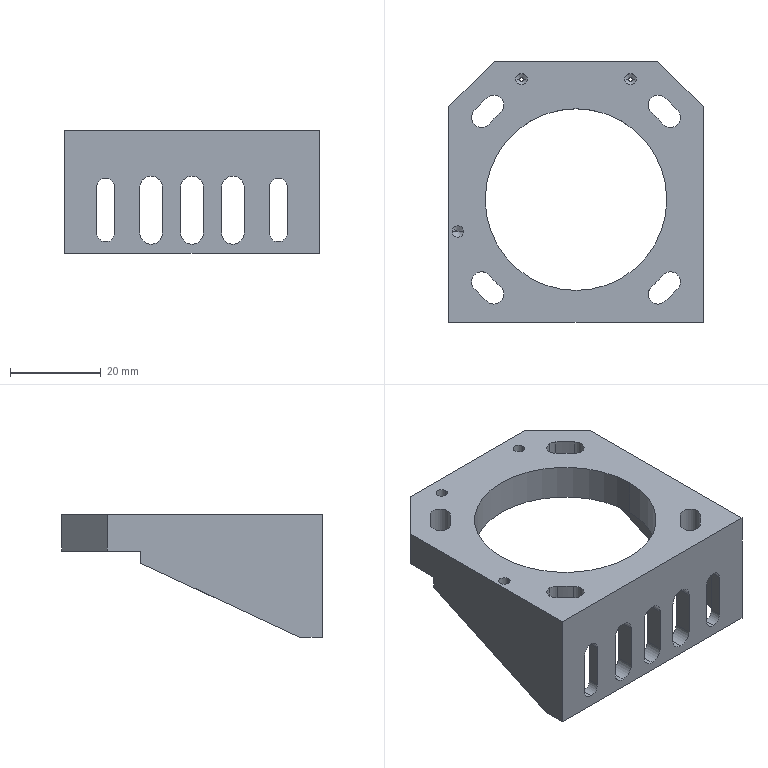NC program | NX | posted with a generic post | part box 56 x 57.4 x 27 mm
Lines 19681 to 20877 of 23725:
(ZLEVEL_PROFILE_COPY_2_COPY_COPY , TOOL : D6R0.5)
N39330 T05 M6
N39332 G54
N39334 G17 G0 G90 X-19.929 Y-23.487 B0. C0. S7000 M3
N39336 G43 Z30. H5
N39338 Z0.958
N39340 G94 G1 Z-0.042 F1000.
N39342 X-20.699 Y-23.932
N39344 G3 X-20.999 Y-24.451 R0.6
N39346 G1 Y-28.473 F3000.
N39348 X-20.953 Y-28.474 Z-0.063
N39350 X-20.909 Z-0.085
N39352 X-20.908 Y-28.
N39354 Y-24.969
N39356 Y-24.456
N39358 X-20.863 Y-24.459 Z-0.106
N39360 X-20.818 Y-24.461 Z-0.127
N39362 X-20.817 Y-24.98
N39364 Y-28.
N39366 X-20.818 Y-28.475
N39368 X-20.772 Z-0.148
N39370 X-20.727 Z-0.169
N39372 Y-28.
N39374 Y-24.99
N39376 Y-24.464
N39378 X-20.681 Y-24.466 Z-0.19
N39380 X-20.637 Y-24.467 Z-0.211
N39382 X-20.636 Y-24.994
N39384 Y-28.
N39386 X-20.637 Y-28.476
N39388 X-20.591 Z-0.232
N39390 X-20.546 Z-0.254
N39392 X-20.545 Y-28.
N39394 Y-24.998
N39396 X-20.546 Y-24.47
N39398 X-20.5 Y-24.471 Z-0.275
N39400 X-20.455 Y-24.472 Z-0.296
N39402 Y-25.
N39404 Y-28.
N39406 Y-28.477
N39408 X-20.409 Z-0.317
N39410 X-20.365 Y-28.478 Z-0.338
N39412 X-20.364 Y-28.
N39414 Y-25.
N39416 X-20.365 Y-24.473
N39418 X-20.319 Y-24.474 Z-0.359
N39420 X-20.274 Z-0.38
N39422 X-20.273 Y-25.
N39424 Y-28.
N39426 X-20.274 Y-28.478
N39428 X-20.228 Z-0.401
N39430 X-20.184 Y-28.479 Z-0.423
N39432 X-20.183 Y-28.
N39434 Y-25.
N39436 X-20.184 Y-24.475
N39438 X-20.138 Z-0.444
N39440 X-20.093 Z-0.465
N39442 X-20.092 Y-25.
N39444 Y-28.
N39446 X-20.093 Y-28.479
N39448 X-20.047 Y-28.48 Z-0.486
N39450 X-20.002 Z-0.507
N39452 Y-28.
N39454 Y-25.
N39456 Y-24.476
N39458 X-19.956 Y-24.477 Z-0.528
N39460 X-19.912 Z-0.549
N39462 X-19.911 Y-25.
N39464 Y-28.
N39466 X-19.912 Y-28.48
N39468 X-19.866 Y-28.481 Z-0.571
N39470 X-19.821 Z-0.592
N39472 X-19.82 Y-28.
N39474 Y-25.
N39476 X-19.821 Y-24.478
N39478 X-19.775 Z-0.613
N39480 X-19.731 Z-0.634
N39482 X-19.73 Y-25.
N39484 Y-28.
N39486 Y-28.482
N39488 X-19.684 Z-0.655
N39490 X-19.64 Z-0.676
N39492 X-19.639 Y-28.
N39494 Y-25.
N39496 X-19.64 Y-24.479
N39498 X-19.594 Y-24.48 Z-0.697
N39500 X-19.549 Z-0.718
N39502 X-19.548 Y-25.
N39504 Y-28.
N39506 X-19.549 Y-28.483
N39508 X-19.503 Z-0.74
N39510 X-19.458 Z-0.761
N39512 Y-28.
N39514 Y-25.
N39516 X-19.459 Y-24.481
N39518 X-19.412 Z-0.782
N39520 X-19.368 Z-0.803
N39522 X-19.367 Y-25.
N39524 Y-28.
N39526 X-19.368 Y-28.484
N39528 X-19.322 Z-0.824
N39530 X-19.277 Z-0.845
N39532 Y-28.
N39534 Y-25.
N39536 Y-24.482
N39538 X-19.231 Z-0.866
N39540 X-19.187 Y-24.483 Z-0.887
N39542 X-19.186 Y-25.
N39544 Y-28.
N39546 Y-28.485
N39548 X-19.141 Z-0.909
N39550 X-19.096 Z-0.93
N39552 X-19.095 Y-28.
N39554 Y-25.
N39556 X-19.096 Y-24.483
N39558 X-19.05 Y-24.484 Z-0.951
N39560 X-19.006 Z-0.972
N39562 X-19.005 Y-25.
N39564 Y-28.
N39566 Y-28.486
N39568 X-18.959 Z-0.993
N39570 X-18.915 Z-1.014
N39572 X-18.914 Y-28.
N39574 Y-25.
N39576 X-18.915 Y-24.485
N39578 X-18.869 Z-1.035
N39580 X-18.824 Y-24.486 Z-1.057
N39582 X-18.823 Y-25.
N39584 Y-28.
N39586 X-18.824 Y-28.487
N39588 X-18.778 Z-1.078
N39590 X-18.733 Z-1.099
N39592 Y-28.
N39594 Y-25.
N39596 X-18.734 Y-24.486
N39598 X-18.687 Z-1.12
N39600 X-18.643 Y-24.487 Z-1.141
N39602 X-18.642 Y-25.
N39604 Y-28.
N39606 X-18.643 Y-28.487
N39608 X-18.597 Y-28.488 Z-1.162
N39610 X-18.552 Z-1.183
N39612 X-18.551 Y-28.
N39614 Y-25.
N39616 X-18.553 Y-24.487
N39618 X-18.506 Z-1.204
N39620 X-18.462 Z-1.226
N39622 X-18.461 Y-25.
N39624 Y-28.
N39626 Y-28.488
N39628 X-18.416 Y-28.489 Z-1.247
N39630 X-18.371 Z-1.268
N39632 X-18.37 Y-28.
N39634 Y-25.
N39636 X-18.371 Y-24.488
N39638 X-18.325 Z-1.289
N39640 X-18.281 Z-1.31
N39642 X-18.28 Y-25.
N39644 Y-28.
N39646 Y-28.489
N39648 X-18.234 Z-1.331
N39650 X-18.189 Y-28.49 Z-1.352
N39652 Y-28.
N39654 Y-25.
N39656 X-18.19 Y-24.489
N39658 X-18.144 Z-1.374
N39660 X-18.099 Z-1.395
N39662 X-18.098 Y-25.
N39664 Y-28.
N39666 X-18.099 Y-28.49
N39668 X-18.053 Z-1.416
N39670 X-18.008 Y-28.491 Z-1.437
N39672 Y-28.
N39674 Y-25.
N39676 X-18.009 Y-24.49
N39678 X-17.962 Z-1.458
N39680 X-17.918 Z-1.479
N39682 X-17.917 Y-25.
N39684 Y-28.
N39686 X-17.918 Y-28.491
N39688 X-17.872 Z-1.5
N39690 X-17.827 Z-1.521
N39692 X-17.826 Y-28.
N39694 Y-25.
N39696 X-17.828 Y-24.49
N39698 X-17.781 Y-24.491 Z-1.543
N39700 X-17.737 Z-1.564
N39702 X-17.736 Y-25.
N39704 Y-28.
N39706 Y-28.492
N39708 X-17.69 Z-1.585
N39710 X-17.646 Z-1.606
N39712 X-17.645 Y-28.
N39714 Y-25.
N39716 X-17.646 Y-24.491
N39718 X-17.6 Z-1.627
N39720 X-17.556 Y-24.492 Z-1.648
N39722 X-17.555 Y-25.
N39724 Y-28.
N39726 Y-28.493
N39728 X-17.509 Z-1.669
N39730 X-17.464 Z-1.69
N39732 Y-28.
N39734 Y-25.
N39736 X-17.465 Y-24.492
N39738 X-17.419 Z-1.712
N39740 X-17.374 Z-1.733
N39742 X-17.373 Y-25.
N39744 Y-28.
N39746 X-17.374 Y-28.493
N39748 X-17.328 Z-1.754
N39750 X-17.283 Z-1.775
N39752 Y-28.
N39754 Y-25.
N39756 X-17.284 Y-24.493
N39758 X-17.237 Z-1.796
N39760 X-17.193 Z-1.817
N39762 X-17.192 Y-25.
N39764 Y-28.
N39766 Y-28.494
N39768 X-17.147 Z-1.838
N39770 X-17.102 Z-1.86
N39772 X-17.101 Y-28.
N39774 Y-25.
N39776 X-17.103 Y-24.494
N39778 X-17.056 Z-1.881
N39780 X-17.012 Z-1.902
N39782 X-17.011 Y-25.
N39784 Y-28.
N39786 Y-28.494
N39788 X-16.965 Z-1.923
N39790 X-16.921 Z-1.944
N39792 X-16.92 Y-28.
N39794 Y-25.
N39796 X-16.921 Y-24.494
N39798 X-16.875 Z-1.965
N39800 X-16.831 Y-24.495 Z-1.986
N39802 X-16.83 Y-25.
N39804 Y-28.
N39806 Y-28.495
N39808 X-16.784 Z-2.007
N39810 X-16.739 Z-2.029
N39812 Y-28.
N39814 Y-25.
N39816 X-16.74 Y-24.495
N39818 X-16.694 Z-2.05
N39820 X-16.649 Z-2.071
N39822 X-16.648 Y-25.
N39824 Y-28.
N39826 X-16.649 Y-28.495
N39828 X-16.603 Z-2.092
N39830 X-16.558 Z-2.113
N39832 Y-28.
N39834 Y-25.
N39836 X-16.559 Y-24.495
N39838 X-16.512 Z-2.134
N39840 X-16.468 Z-2.155
N39842 X-16.467 Y-25.
N39844 Y-28.
N39846 Y-28.495
N39848 X-16.422 Z-2.176
N39850 X-16.377 Y-28.496 Z-2.198
N39852 X-16.376 Y-28.
N39854 Y-25.
N39856 X-16.378 Y-24.495
N39858 X-16.331 Y-24.496 Z-2.219
N39860 X-16.287 Z-2.24
N39862 X-16.286 Y-25.
N39864 Y-28.
N39866 Y-28.496
N39868 X-16.24 Z-2.261
N39870 X-16.196 Z-2.282
N39872 X-16.195 Y-28.
N39874 Y-25.
N39876 X-16.196 Y-24.496
N39878 X-16.15 Z-2.303
N39880 X-16.106 Z-2.324
N39882 X-16.104 Y-25.
N39884 Y-28.
N39886 X-16.105 Y-28.496
N39888 X-16.059 Z-2.346
N39890 X-16.014 Y-28.497 Z-2.367
N39892 Y-28.
N39894 Y-25.
N39896 X-16.015 Y-24.496
N39898 X-15.969 Y-24.497 Z-2.388
N39900 X-15.924 Z-2.409
N39902 X-15.923 Y-25.
N39904 Y-28.
N39906 X-15.924 Y-28.497
N39908 X-15.878 Z-2.43
N39910 X-15.833 Z-2.451
N39912 Y-28.
N39914 Y-25.
N39916 X-15.834 Y-24.497
N39918 X-15.787 Z-2.472
N39920 X-15.743 Z-2.493
N39922 X-15.742 Y-25.
N39924 Y-28.
N39926 Y-28.497
N39928 X-15.697 Z-2.515
N39930 X-15.652 Z-2.536
N39932 X-15.651 Y-28.
N39934 Y-25.
N39936 X-15.653 Y-24.497
N39938 X-15.606 Z-2.557
N39940 X-15.562 Z-2.578
N39942 X-15.561 Y-25.
N39944 Y-28.
N39946 Y-28.497
N39948 X-15.515 Z-2.599
N39950 X-15.47 Z-2.62
N39952 Y-28.
N39954 Y-25.
N39956 X-15.471 Y-24.498
N39958 X-15.425 Z-2.641
N39960 X-15.381 Z-2.662
N39962 X-15.379 Y-25.
N39964 Y-28.
N39966 X-15.38 Y-28.498
N39968 X-15.334 Z-2.684
N39970 X-15.289 Z-2.705
N39972 Y-28.
N39974 Y-25.
N39976 X-15.29 Y-24.498
N39978 X-15.243 Z-2.726
N39980 X-15.199 Z-2.747
N39982 X-15.198 Y-25.
N39984 Y-28.
N39986 X-15.199 Y-28.498
N39988 X-15.153 Z-2.768
N39990 X-15.108 Z-2.789
N39992 Y-28.
N39994 Y-25.
N39996 X-15.109 Y-24.498
N39998 X-15.062 Z-2.81
N40000 X-15.018 Z-2.832
N40002 X-15.017 Y-25.
N40004 Y-28.
N40006 Y-28.498
N40008 X-14.972 Z-2.853
N40010 X-14.927 Z-2.874
N40012 X-14.926 Y-28.
N40014 Y-25.
N40016 X-14.927 Y-24.498
N40018 X-14.881 Z-2.895
N40020 X-14.837 Z-2.916
N40022 X-14.836 Y-25.
N40024 Y-28.
N40026 Y-28.498
N40028 X-14.79 Z-2.937
N40030 X-14.745 Z-2.958
N40032 Y-28.
N40034 Y-25.
N40036 X-14.746 Y-24.498
N40038 X-14.7 Z-2.979
N40040 X-14.656 Z-3.001
N40042 X-14.654 Y-25.
N40044 Y-28.
N40046 X-14.655 Y-28.498
N40048 X-14.609 Z-3.022
N40050 X-14.564 Z-3.043
N40052 Y-28.
N40054 Y-25.
N40056 X-14.565 Y-24.499
N40058 X-14.518 Z-3.064
N40060 X-14.474 Z-3.085
N40062 X-14.473 Y-25.
N40064 Y-28.
N40066 Y-28.498
N40068 X-14.428 Y-28.499 Z-3.106
N40070 X-14.383 Z-3.127
N40072 X-14.382 Y-28.
N40074 Y-25.
N40076 X-14.384 Y-24.499
N40078 X-14.337 Z-3.149
N40080 X-14.293 Z-3.17
N40082 X-14.292 Y-25.
N40084 Y-28.
N40086 Y-28.499
N40088 X-14.247 Z-3.191
N40090 X-14.202 Z-3.212
N40092 X-14.201 Y-28.
N40094 Y-25.
N40096 X-14.202 Y-24.499
N40098 X-14.156 Z-3.233
N40100 X-14.112 Z-3.254
N40102 X-14.111 Y-25.
N40104 Y-28.
N40106 Y-28.499
N40108 X-14.065 Z-3.275
N40110 X-14.02 Z-3.296
N40112 Y-28.
N40114 Y-25.
N40116 X-14.021 Y-24.499
N40118 X-13.975 Z-3.318
N40120 X-13.931 Z-3.339
N40122 X-13.929 Y-25.
N40124 Y-28.
N40126 X-13.93 Y-28.499
N40128 X-13.884 Z-3.36
N40130 X-13.839 Z-3.381
N40132 Y-28.
N40134 Y-25.
N40136 X-13.84 Y-24.499
N40138 X-13.793 Z-3.402
N40140 X-13.749 Z-3.423
N40142 X-13.748 Y-25.
N40144 Y-28.
N40146 Y-28.499
N40148 X-13.703 Z-3.444
N40150 X-13.658 Z-3.465
N40152 X-13.657 Y-28.
N40154 Y-25.
N40156 X-13.659 Y-24.499
N40158 X-13.612 Z-3.487
N40160 X-13.568 Z-3.508
N40162 X-13.567 Y-25.
N40164 Y-28.
N40166 Y-28.499
N40168 X-13.521 Z-3.529
N40170 X-13.477 Z-3.55
N40172 X-13.476 Y-28.
N40174 Y-25.
N40176 X-13.477 Y-24.499
N40178 X-13.431 Z-3.571
N40180 X-13.387 Z-3.592
N40182 X-13.386 Y-25.
N40184 Y-28.
N40186 Y-28.499
N40188 X-13.34 Z-3.613
N40190 X-13.295 Z-3.635
N40192 Y-28.
N40194 Y-25.
N40196 X-13.296 Y-24.499
N40198 X-13.25 Z-3.656
N40200 X-13.206 Y-24.5 Z-3.677
N40202 X-13.204 Y-25.
N40204 Y-28.
N40206 X-13.205 Y-28.499
N40208 X-13.159 Z-3.698
N40210 X-13.114 Z-3.719
N40212 Y-28.
N40214 Y-25.
N40216 X-13.115 Y-24.5
N40218 X-13.068 Z-3.74
N40220 X-13.024 Z-3.761
N40222 X-13.023 Y-25.
N40224 Y-28.
N40226 Y-28.499
N40228 X-12.978 Z-3.782
N40230 X-12.933 Z-3.804
N40232 X-12.932 Y-28.
N40234 Y-25.
N40236 X-12.934 Y-24.5
N40238 X-12.887 Z-3.825
N40240 X-12.843 Z-3.846
N40242 X-12.842 Y-25.
N40244 Y-28.
N40246 Y-28.499
N40248 X-12.796 Z-3.867
N40250 X-12.751 Z-3.888
N40252 Y-28.
N40254 Y-25.
N40256 X-12.752 Y-24.5
N40258 X-12.706 Z-3.909
N40260 X-12.662 Z-3.93
N40262 X-12.66 Y-25.
N40264 Y-28.
N40266 X-12.661 Y-28.5
N40268 X-12.615 Z-3.951
N40270 X-12.57 Z-3.973
N40272 Y-28.
N40274 Y-25.
N40276 X-12.571 Y-24.5
N40278 X-12.525 Z-3.994
N40280 X-12.48 Z-4.015
N40282 X-12.479 Y-25.
N40284 Y-28.
N40286 X-12.48 Y-28.5
N40288 X-12.434 Z-4.036
N40290 X-12.389 Z-4.057
N40292 Y-28.
N40294 Y-25.
N40296 X-12.39 Y-24.5
N40298 X-12.343 Z-4.078
N40300 X-12.299 Z-4.099
N40302 X-12.298 Y-25.
N40304 Y-28.
N40306 Y-28.5
N40308 X-12.253 Z-4.121
N40310 X-12.208 Z-4.142
N40312 X-12.207 Y-28.
N40314 Y-25.
N40316 X-12.209 Y-24.5
N40318 X-12.162 Z-4.163
N40320 X-12.118 Z-4.184
N40322 X-12.117 Y-25.
N40324 Y-28.
N40326 Y-28.5
N40328 X-12.071 Z-4.205
N40330 X-12.026 Z-4.226
N40332 Y-28.
N40334 Y-25.
N40336 X-12.027 Y-24.5
N40338 X-11.981 Z-4.247
N40340 X-11.937 Z-4.268
N40342 X-11.935 Y-25.
N40344 Y-28.
N40346 X-11.936 Y-28.5
N40348 X-11.89 Z-4.29
N40350 X-11.845 Z-4.311
N40352 Y-28.
N40354 Y-25.
N40356 X-11.846 Y-24.5
N40358 X-11.799 Z-4.332
N40360 X-11.755 Z-4.353
N40362 X-11.754 Y-25.
N40364 Y-28.
N40366 X-11.755 Y-28.5
N40368 X-11.709 Z-4.374
N40370 X-11.664 Z-4.395
N40372 Y-28.
N40374 Y-25.
N40376 X-11.665 Y-24.5
N40378 X-11.618 Z-4.416
N40380 X-11.574 Z-4.437
N40382 X-11.573 Y-25.
N40384 Y-28.
N40386 Y-28.5
N40388 X-11.528 Z-4.459
N40390 X-11.483 Z-4.48
N40392 X-11.482 Y-28.
N40394 Y-25.
N40396 X-11.484 Y-24.5
N40398 X-11.437 Z-4.501
N40400 X-11.393 Z-4.522
N40402 X-11.392 Y-25.
N40404 Y-28.
N40406 Y-28.5
N40408 X-11.346 Z-4.543
N40410 X-11.301 Z-4.564
N40412 Y-28.
N40414 Y-25.
N40416 X-11.302 Y-24.5
N40418 X-11.256 Z-4.585
N40420 X-11.212 Z-4.607
N40422 X-11.21 Y-25.
N40424 Y-28.
N40426 X-11.211 Y-28.5
N40428 X-11.165 Z-4.628
N40430 X-11.12 Z-4.649
N40432 Y-28.
N40434 Y-25.
N40436 X-11.121 Y-24.5
N40438 X-11.074 Z-4.67
N40440 X-11.03 Z-4.691
N40442 X-11.029 Y-25.
N40444 Y-28.
N40446 Y-28.5
N40448 X-10.984 Z-4.712
N40450 X-10.939 Z-4.733
N40452 Y-28.
N40454 Y-25.
N40456 X-10.94 Y-24.5
N40458 X-10.893 Z-4.754
N40460 X-10.849 Z-4.776
N40462 X-10.848 Y-25.
N40464 Y-28.
N40466 Y-28.5
N40468 X-10.803 Z-4.797
N40470 X-10.758 Z-4.818
N40472 X-10.757 Y-28.
N40474 Y-25.
N40476 X-10.759 Y-24.5
N40478 X-10.712 Z-4.839
N40480 X-10.668 Z-4.86
N40482 X-10.667 Y-25.
N40484 Y-28.
N40486 Y-28.5
N40488 X-10.621 Z-4.881
N40490 X-10.576 Z-4.902
N40492 Y-28.
N40494 Y-25.
N40496 X-10.577 Y-24.5
N40498 X-10.531 Z-4.924
N40500 X-10.487 Z-4.945
N40502 X-10.485 Y-25.
N40504 Y-28.
N40506 X-10.486 Y-28.5
N40508 X-10.44 Z-4.966
N40510 X-10.395 Z-4.987
N40512 Y-28.
N40514 Y-25.
N40516 X-10.396 Y-24.5
N40518 X-10.349 Z-5.008
N40520 X-10.305 Z-5.029
N40522 X-10.304 Y-25.
N40524 Y-28.
N40526 Y-28.5
N40528 X-10.259 Z-5.05
N40530 X-10.214 Z-5.071
N40532 X-10.213 Y-28.
N40534 Y-25.
N40536 X-10.215 Y-24.5
N40538 X-10.168 Z-5.093
N40540 X-10.124 Z-5.114
N40542 X-10.123 Y-25.
N40544 Y-28.
N40546 Y-28.5
N40548 X-10.078 Z-5.135
N40550 X-10.033 Z-5.156
N40552 X-10.032 Y-28.
N40554 Y-25.
N40556 X-10.033 Y-24.5
N40558 X-9.987 Z-5.177
N40560 X-9.943 Z-5.198
N40562 X-9.942 Y-25.
N40564 Y-28.
N40566 Y-28.5
N40568 X-9.896 Z-5.219
N40570 X-9.851 Z-5.24
N40572 Y-28.
N40574 Y-25.
N40576 X-9.852 Y-24.5
N40578 X-9.806 Z-5.262
N40580 X-9.762 Z-5.283
N40582 X-9.76 Y-25.
N40584 Y-28.
N40586 X-9.761 Y-28.5
N40588 X-9.715 Z-5.304
N40590 X-9.67 Z-5.325
N40592 Y-28.
N40594 Y-25.
N40596 X-9.671 Y-24.5
N40598 X-9.624 Z-5.346
N40600 X-9.58 Z-5.367
N40602 X-9.579 Y-25.
N40604 Y-28.
N40606 Y-28.5
N40608 X-9.534 Z-5.388
N40610 X-9.489 Z-5.41
N40612 X-9.488 Y-28.
N40614 Y-25.
N40616 X-9.49 Y-24.5
N40618 X-9.443 Z-5.431
N40620 X-9.399 Z-5.452
N40622 X-9.398 Y-25.
N40624 Y-28.
N40626 Y-28.5
N40628 X-9.352 Z-5.473
N40630 X-9.308 Z-5.494
N40632 X-9.307 Y-28.
N40634 Y-25.
N40636 X-9.308 Y-24.5
N40638 X-9.262 Z-5.515
N40640 X-9.218 Z-5.536
N40642 X-9.217 Y-25.
N40644 Y-28.
N40646 Y-28.5
N40648 X-9.171 Z-5.557
N40650 X-9.126 Z-5.579
N40652 Y-28.
N40654 Y-25.
N40656 Y-24.5
N40658 X-9.081 Z-5.6
N40660 X-9.037 Z-5.621
N40662 X-9.035 Y-25.
N40664 Y-28.
N40666 X-9.036 Y-28.5
N40668 X-8.99 Z-5.642
N40670 X-8.945 Z-5.663
N40672 Y-28.
N40674 Y-25.
N40676 X-8.946 Y-24.5
N40678 X-8.899 Z-5.684
N40680 X-8.855 Z-5.705
N40682 X-8.854 Y-25.
N40684 Y-28.
N40686 Y-28.5
N40688 X-8.809 Z-5.726
N40690 X-8.764 Z-5.748
N40692 X-8.763 Y-28.
N40694 Y-25.
N40696 X-8.765 Y-24.5
N40698 X-8.718 Z-5.769
N40700 X-8.674 Z-5.79
N40702 X-8.673 Y-25.
N40704 Y-28.
N40706 Y-28.5
N40708 X-8.627 Z-5.811
N40710 X-8.582 Z-5.832
N40712 Y-28.
N40714 Y-25.
N40716 X-8.583 Y-24.5
N40718 X-8.537 Z-5.853
N40720 X-8.493 Z-5.874
N40722 X-8.491 Y-25.
N40724 Y-28.
N40726 X-8.492 Y-28.5
N40728 X-8.446 Z-5.896
N40730 X-8.401 Z-5.917
N40732 Y-28.
N40734 Y-25.
N40736 X-8.402 Y-24.5
N40738 X-8.356 Z-5.938
N40740 X-8.311 Z-5.959
N40742 X-8.31 Y-25.
N40744 Y-28.
N40746 X-8.311 Y-28.5
N40748 X-8.265 Z-5.98
N40750 X-8.22 Z-6.001
N40752 Y-28.
N40754 Y-25.
N40756 X-8.221 Y-24.5
N40758 X-8.174 Z-6.022
N40760 X-8.13 Z-6.043
N40762 X-8.129 Y-25.
N40764 Y-28.
N40766 Y-28.5
N40768 X-8.084 Z-6.065
N40770 X-8.039 Z-6.086
N40772 X-8.038 Y-28.
N40774 Y-25.
N40776 X-8.04 Y-24.5
N40778 X-7.993 Z-6.107
N40780 X-7.949 Z-6.128
N40782 X-7.948 Y-25.
N40784 Y-28.
N40786 Y-28.5
N40788 X-7.902 Z-6.149
N40790 X-7.857 Z-6.17
N40792 Y-28.
N40794 Y-25.
N40796 X-7.858 Y-24.5
N40798 X-7.812 Z-6.191
N40800 X-7.768 Z-6.212
N40802 X-7.766 Y-25.
N40804 Y-28.
N40806 X-7.767 Y-28.5
N40808 X-7.721 Z-6.234
N40810 X-7.676 Z-6.255
N40812 Y-28.
N40814 Y-25.
N40816 X-7.677 Y-24.5
N40818 X-7.63 Z-6.276
N40820 X-7.586 Z-6.297
N40822 X-7.585 Y-25.
N40824 Y-28.
N40826 X-7.586 Y-28.5
N40828 X-7.54 Z-6.318
N40830 X-7.495 Z-6.339
N40832 Y-28.
N40834 Y-25.
N40836 X-7.496 Y-24.5
N40838 X-7.449 Z-6.36
N40840 X-7.405 Z-6.382
N40842 X-7.404 Y-25.
N40844 Y-28.
N40846 Y-28.5
N40848 X-7.359 Z-6.403
N40850 X-7.314 Z-6.424
N40852 X-7.313 Y-28.
N40854 Y-25.
N40856 X-7.315 Y-24.5
N40858 X-7.268 Z-6.445
N40860 X-7.224 Z-6.466
N40862 X-7.223 Y-25.
N40864 Y-28.
N40866 Y-28.5
N40868 X-7.177 Z-6.487
N40870 X-7.132 Z-6.508
N40872 Y-28.
N40874 Y-25.
N40876 X-7.133 Y-24.5
N40878 X-7.087 Z-6.529
N40880 X-7.043 Z-6.551
N40882 X-7.041 Y-25.
N40884 Y-28.
N40886 X-7.042 Y-28.5
N40888 X-6.996 Z-6.572
N40890 X-6.951 Z-6.593
N40892 Y-28.
N40894 Y-25.
N40896 X-6.952 Y-24.5
N40898 X-6.905 Z-6.614
N40900 X-6.861 Z-6.635
N40902 X-6.86 Y-25.
N40904 Y-28.
N40906 Y-28.5
N40908 X-6.815 Z-6.656
N40910 X-6.77 Z-6.677
N40912 X-6.769 Y-28.
N40914 Y-25.
N40916 X-6.771 Y-24.5
N40918 X-6.724 Z-6.699
N40920 X-6.68 Z-6.72
N40922 X-6.679 Y-25.
N40924 Y-28.
N40926 Y-28.5
N40928 X-6.634 Z-6.741
N40930 X-6.589 Z-6.762
N40932 X-6.588 Y-28.
N40934 Y-25.
N40936 X-6.59 Y-24.5
N40938 X-6.543 Z-6.783
N40940 X-6.499 Z-6.804
N40942 X-6.498 Y-25.
N40944 Y-28.
N40946 Y-28.5
N40948 X-6.452 Z-6.825
N40950 X-6.407 Z-6.846
N40952 Y-28.
N40954 Y-25.
N40956 X-6.408 Y-24.5
N40958 X-6.362 Z-6.868
N40960 X-6.318 Z-6.889
N40962 X-6.316 Y-25.
N40964 Y-28.
N40966 X-6.317 Y-28.5
N40968 X-6.271 Z-6.91
N40970 X-6.226 Z-6.931
N40972 Y-28.
N40974 Y-25.
N40976 X-6.227 Y-24.5
N40978 X-6.18 Z-6.952
N40980 X-6.136 Z-6.973
N40982 X-6.135 Y-25.
N40984 Y-28.
N40986 Y-28.5
N40988 X-6.09 Z-6.994
N40990 X-6.045 Z-7.015
N40992 X-6.044 Y-28.
N40994 Y-25.
N40996 X-6.046 Y-24.5
N40998 X-5.999 Z-7.037
N41000 X-5.955 Z-7.058
N41002 X-5.954 Y-25.
N41004 Y-28.
N41006 Y-28.5
N41008 X-5.908 Z-7.079
N41010 X-5.864 Z-7.1
N41012 X-5.863 Y-28.
N41014 Y-25.
N41016 X-5.864 Y-24.5
N41018 X-5.818 Z-7.121
N41020 X-5.774 Z-7.142
N41022 X-5.773 Y-25.
N41024 Y-28.
N41026 Y-28.5
N41028 X-5.727 Z-7.163
N41030 X-5.682 Z-7.185
N41032 Y-28.
N41034 Y-25.
N41036 X-5.683 Y-24.5
N41038 X-5.637 Z-7.206
N41040 X-5.593 Z-7.227
N41042 X-5.591 Y-25.
N41044 Y-28.
N41046 X-5.592 Y-28.5
N41048 X-5.546 Z-7.248
N41050 X-5.501 Z-7.269
N41052 Y-28.
N41054 Y-25.
N41056 X-5.502 Y-24.5
N41058 X-5.455 Z-7.29
N41060 X-5.411 Z-7.311
N41062 X-5.41 Y-25.
N41064 Y-28.
N41066 Y-28.5
N41068 X-5.365 Z-7.332
N41070 X-5.32 Z-7.354
N41072 X-5.319 Y-28.
N41074 Y-25.
N41076 X-5.321 Y-24.5
N41078 X-5.274 Z-7.375
N41080 X-5.23 Z-7.396
N41082 X-5.229 Y-25.
N41084 Y-28.
N41086 Y-28.5
N41088 X-5.183 Z-7.417
N41090 X-5.138 Z-7.438
N41092 Y-28.
N41094 Y-25.
N41096 X-5.139 Y-24.5
N41098 X-5.093 Z-7.459
N41100 X-5.049 Z-7.48
N41102 X-5.048 Y-25.
N41104 Y-28.
N41106 Y-28.5
N41108 X-5.002 Z-7.501
N41110 X-4.957 Z-7.523
N41112 Y-28.
N41114 Y-25.
N41116 X-4.958 Y-24.5
N41118 X-4.912 Z-7.544
N41120 X-4.868 Z-7.565
N41122 X-4.866 Y-25.
N41124 Y-28.
N41126 X-4.867 Y-28.5
N41128 X-4.821 Z-7.586
N41130 X-4.776 Z-7.607
N41132 Y-28.
N41134 Y-25.
N41136 X-4.777 Y-24.5
N41138 X-4.73 Z-7.628
N41140 X-4.686 Z-7.649
N41142 X-4.685 Y-25.
N41144 Y-28.
N41146 Y-28.5
N41148 X-4.64 Z-7.671
N41150 X-4.595 Z-7.692
N41152 X-4.594 Y-28.
N41154 Y-25.
N41156 X-4.596 Y-24.5
N41158 X-4.549 Z-7.713
N41160 X-4.505 Z-7.734
N41162 X-4.504 Y-25.
N41164 Y-28.
N41166 Y-28.5
N41168 X-4.458 Z-7.755
N41170 X-4.413 Z-7.776
N41172 Y-28.
N41174 Y-25.
N41176 X-4.414 Y-24.5
N41178 X-4.368 Z-7.797
N41180 X-4.324 Z-7.818
N41182 X-4.322 Y-25.
N41184 Y-28.
N41186 X-4.323 Y-28.5
N41188 X-4.277 Z-7.84
N41190 X-4.232 Z-7.861
N41192 Y-28.
N41194 Y-25.
N41196 X-4.233 Y-24.5
N41198 X-4.187 Z-7.882
N41200 X-4.142 Z-7.903
N41202 X-4.141 Y-25.
N41204 Y-28.
N41206 X-4.142 Y-28.5
N41208 X-4.096 Z-7.924
N41210 X-4.051 Z-7.945
N41212 Y-28.
N41214 Y-25.
N41216 X-4.052 Y-24.5
N41218 X-4.005 Z-7.966
N41220 X-3.961 Z-7.987
N41222 X-3.96 Y-25.
N41224 Y-28.
N41226 Y-28.5
N41228 X-3.915 Z-8.009
N41230 X-3.87 Z-8.03
N41232 X-3.869 Y-28.
N41234 Y-25.
N41236 X-3.871 Y-24.5
N41238 X-3.824 Z-8.051
N41240 X-3.78 Z-8.072
N41242 X-3.779 Y-25.
N41244 Y-28.
N41246 Y-28.5
N41248 X-3.733 Z-8.093
N41250 X-3.688 Z-8.114
N41252 Y-28.
N41254 Y-25.
N41256 X-3.689 Y-24.5
N41258 X-3.643 Z-8.135
N41260 X-3.599 Z-8.157
N41262 X-3.597 Y-25.
N41264 Y-28.
N41266 X-3.598 Y-28.5
N41268 X-3.552 Z-8.178
N41270 X-3.507 Z-8.199
N41272 Y-28.
N41274 Y-25.
N41276 X-3.508 Y-24.5
N41278 X-3.461 Z-8.22
N41280 X-3.417 Z-8.241
N41282 X-3.416 Y-25.
N41284 Y-28.
N41286 X-3.417 Y-28.5
N41288 X-3.371 Z-8.262
N41290 X-3.326 Z-8.283
N41292 Y-28.
N41294 Y-25.
N41296 X-3.327 Y-24.5
N41298 X-3.28 Z-8.304
N41300 X-3.236 Z-8.326
N41302 X-3.235 Y-25.
N41304 Y-28.
N41306 Y-28.5
N41308 X-3.19 Z-8.347
N41310 X-3.145 Z-8.368
N41312 X-3.144 Y-28.
N41314 Y-25.
N41316 X-3.146 Y-24.5
N41318 X-3.099 Z-8.389
N41320 X-3.055 Z-8.41
N41322 X-3.054 Y-25.
N41324 Y-28.
N41326 Y-28.5
N41328 X-3.008 Z-8.431
N41330 X-2.963 Z-8.452
N41332 Y-28.
N41334 Y-25.
N41336 X-2.964 Y-24.5
N41338 X-2.918 Z-8.473
N41340 X-2.874 Z-8.495
N41342 X-2.872 Y-25.
N41344 Y-28.
N41346 X-2.873 Y-28.5
N41348 X-2.827 Z-8.516
N41350 X-2.782 Z-8.537
N41352 Y-28.
N41354 Y-25.
N41356 X-2.783 Y-24.5
N41358 X-2.736 Z-8.558
N41360 X-2.692 Z-8.579
N41362 X-2.691 Y-25.
N41364 Y-28.
N41366 Y-28.5
N41368 X-2.646 Z-8.6
N41370 X-2.601 Z-8.621
N41372 X-2.6 Y-28.
N41374 Y-25.
N41376 X-2.602 Y-24.5
N41378 X-2.555 Z-8.643
N41380 X-2.511 Z-8.664
N41382 X-2.51 Y-25.
N41384 Y-28.
N41386 Y-28.5
N41388 X-2.465 Z-8.685
N41390 X-2.42 Z-8.706
N41392 X-2.419 Y-28.
N41394 Y-25.
N41396 X-2.42 Y-24.5
N41398 X-2.374 Z-8.727
N41400 X-2.33 Z-8.748
N41402 X-2.329 Y-25.
N41404 Y-28.
N41406 Y-28.5
N41408 X-2.283 Z-8.769
N41410 X-2.238 Z-8.79
N41412 Y-28.
N41414 Y-25.
N41416 X-2.239 Y-24.5
N41418 X-2.193 Z-8.812
N41420 X-2.149 Z-8.833
N41422 X-2.147 Y-25.
N41424 Y-28.
N41426 X-2.148 Y-28.5
N41428 X-2.102 Z-8.854
N41430 X-2.057 Z-8.875
N41432 Y-28.
N41434 Y-25.
N41436 X-2.058 Y-24.5
N41438 X-2.011 Z-8.896
N41440 X-1.967 Z-8.917
N41442 X-1.966 Y-25.
N41444 Y-28.
N41446 Y-28.5
N41448 X-1.921 Z-8.938
N41450 X-1.876 Z-8.96
N41452 X-1.875 Y-28.
N41454 Y-25.
N41456 X-1.877 Y-24.5
N41458 X-1.83 Z-8.981
N41460 X-1.786 Z-9.002
N41462 X-1.785 Y-25.
N41464 Y-28.
N41466 Y-28.5
N41468 X-1.739 Z-9.023
N41470 X-1.695 Z-9.044
N41472 X-1.694 Y-28.
N41474 Y-25.
N41476 X-1.695 Y-24.5
N41478 X-1.649 Z-9.065
N41480 X-1.605 Z-9.086
N41482 X-1.604 Y-25.
N41484 Y-28.
N41486 Y-28.5
N41488 X-1.558 Z-9.107
N41490 X-1.513 Z-9.129
N41492 Y-28.
N41494 Y-25.
N41496 X-1.514 Y-24.5
N41498 X-1.468 Z-9.15
N41500 X-1.424 Z-9.171
N41502 X-1.422 Y-25.
N41504 Y-28.
N41506 X-1.423 Y-28.5
N41508 X-1.377 Z-9.192
N41510 X-1.332 Z-9.213
N41512 Y-28.
N41514 Y-25.
N41516 X-1.333 Y-24.5
N41518 X-1.286 Z-9.234
N41520 X-1.242 Z-9.255
N41522 X-1.241 Y-25.
N41524 Y-28.
N41526 Y-28.5
N41528 X-1.196 Z-9.276
N41530 X-1.151 Z-9.298
N41532 X-1.15 Y-28.
N41534 Y-25.
N41536 X-1.152 Y-24.5
N41538 X-1.105 Z-9.319
N41540 X-1.061 Z-9.34
N41542 X-1.06 Y-25.
N41544 Y-28.
N41546 Y-28.5
N41548 X-1.014 Z-9.361
N41550 X-0.969 Z-9.382
N41552 Y-28.
N41554 Y-25.
N41556 X-0.97 Y-24.5
N41558 X-0.924 Z-9.403
N41560 X-0.88 Z-9.424
N41562 X-0.878 Y-25.
N41564 Y-28.
N41566 X-0.879 Y-28.5
N41568 X-0.833 Z-9.446
N41570 X-0.788 Z-9.467
N41572 Y-28.
N41574 Y-25.
N41576 X-0.789 Y-24.5
N41578 X-0.743 Z-9.488
N41580 X-0.698 Z-9.509
N41582 X-0.697 Y-25.
N41584 Y-28.
N41586 X-0.698 Y-28.5
N41588 X-0.652 Z-9.53
N41590 X-0.607 Z-9.551
N41592 Y-28.
N41594 Y-25.
N41596 X-0.608 Y-24.5
N41598 X-0.561 Z-9.572
N41600 X-0.517 Z-9.593
N41602 X-0.516 Y-25.
N41604 Y-28.
N41606 Y-28.5
N41608 X-0.471 Z-9.615
N41610 X-0.426 Z-9.636
N41612 X-0.425 Y-28.
N41614 Y-25.
N41616 X-0.427 Y-24.5
N41618 X-0.38 Z-9.657
N41620 X-0.336 Z-9.678
N41622 X-0.335 Y-25.
N41624 Y-28.
N41626 Y-28.5
N41628 X-0.289 Z-9.699
N41630 X-0.244 Z-9.72
N41632 Y-28.
N41634 Y-25.
N41636 X-0.245 Y-24.5
N41638 X-0.199 Z-9.741
N41640 X-0.155 Z-9.762
N41642 X-0.153 Y-25.
N41644 Y-28.
N41646 X-0.154 Y-28.5
N41648 X-0.108 Z-9.784
N41650 X-0.063 Z-9.805
N41652 Y-28.
N41654 Y-25.
N41656 X-0.064 Y-24.5
N41658 X-0.017 Z-9.826
N41660 X0.027 Z-9.847
N41662 X0.028 Y-25.
N41664 Y-28.
N41666 X0.027 Y-28.5
N41668 X0.073 Z-9.868
N41670 X0.118 Z-9.889
N41672 Y-28.
N41674 Y-25.
N41676 X0.117 Y-24.5
N41678 X0.164 Z-9.91
N41680 X0.208 Z-9.932
N41682 X0.209 Y-25.
N41684 Y-28.
N41686 Y-28.5
N41688 X0.254 Z-9.953
N41690 X0.299 Z-9.974
N41692 X0.3 Y-28.
N41694 Y-25.
N41696 X0.298 Y-24.5
N41698 X0.345 Z-9.995
N41700 X0.389 Z-10.016
N41702 X0.39 Y-25.
N41704 Y-28.
N41706 Y-28.5
N41708 X0.436 Z-10.037
N41710 X0.481 Z-10.058
N41712 Y-28.
N41714 Y-25.
N41716 X0.48 Y-24.5